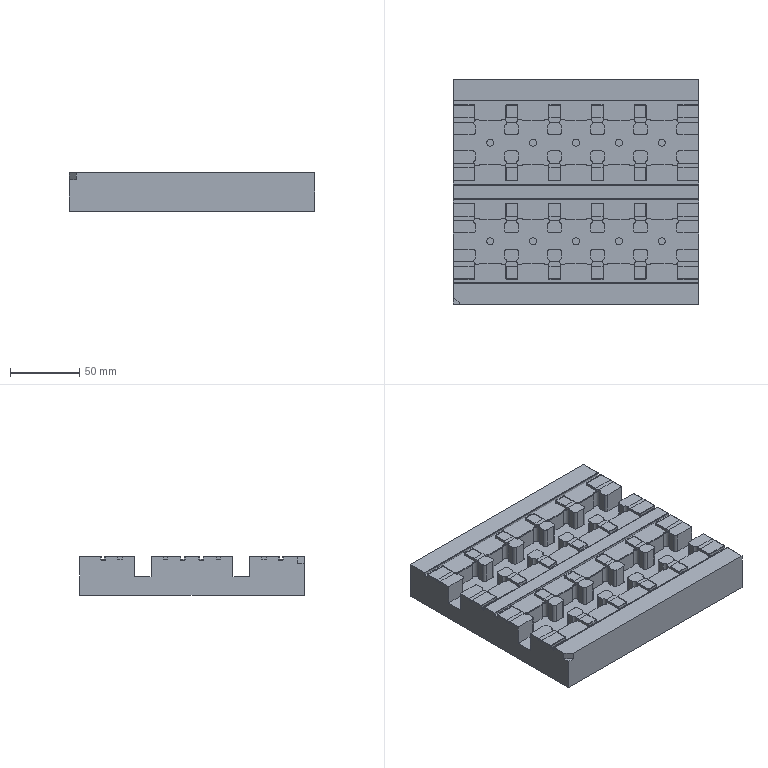NC program | NX | posted by the shop | part box 177 x 162 x 28 mm
Lines 20888 to 21819 of 240480:
N5 T05 M06
(D4  D=4. R=0. H=05 ce=0.02 di=0.05)
(D.N=05 MAX_Z=45. MIN_Z=13.55 Time=44.81M)
T04
G00 G90 G54 X-69.134 Y-48.309 M03 S4000
G43 H05 Z43.
M08
Z28.503
G01 X-69.145 Y-48.308 Z28.405 F1200.
X-69.177 Y-48.307 Z28.318
X-69.229 Y-48.308 Z28.241
X-69.3 Y-48.314 Z28.174
X-69.387 Y-48.328 Z28.115
X-69.49 Y-48.352 Z28.065
X-69.606 Y-48.389 Z28.023
X-69.735 Y-48.44 Z27.988
X-69.875 Y-48.51 Z27.96
X-70.025 Y-48.599 Z27.938
X-70.182 Y-48.712 Z27.922
X-70.346 Y-48.849 Z27.911
X-70.515 Y-49.015 Z27.905
X-70.687 Y-49.211 Z27.903
G02 X-71.571 Y-49.834 I-1.563 J1.28 F1500.
G03 X-71.757 Y-50.097 I.094 J-.264
G01 X-71.753 Y-50.146
G02 X-71.722 Y-50.5 I-1.989 J-.354
X-72.278 Y-51.892 I-2.02 J0.0
X-71.54 Y-53.011 I-1.222 J-1.608
G01 X-71.493 Y-53.158
X-71.436 Y-53.27 Z27.902
X-71.369 Y-53.348 Z27.901
X-71.295 Y-53.395 Z27.9
X-71.214 Y-53.412 Z27.899
X-71.127 Y-53.402 Z27.897
X-71.037 Y-53.366 Z27.895
X-70.942 Y-53.307 Z27.893
X-70.846 Y-53.228 Z27.89
X-70.749 Y-53.129 Z27.888
X-70.652 Y-53.013 Z27.885
X-70.557 Y-52.883 Z27.882
X-70.464 Y-52.74 Z27.879
X-70.376 Y-52.586 Z27.876
X-70.213 Y-52.255 Z27.87
X-70.073 Y-51.898 Z27.864
X-69.957 Y-51.524 Z27.857
X-69.868 Y-51.142 Z27.851
X-69.809 Y-50.759 Z27.844
X-69.78 Y-50.383 Z27.838
X-69.785 Y-50.023 Z27.832
X-69.8 Y-49.852 Z27.829
X-69.825 Y-49.689 Z27.826
X-69.857 Y-49.537 Z27.823
X-69.898 Y-49.398 Z27.82
X-69.946 Y-49.274 Z27.818
X-70.002 Y-49.167 Z27.816
X-70.065 Y-49.08 Z27.813
X-70.136 Y-49.015 Z27.811
X-70.213 Y-48.974 Z27.81
X-70.296 Y-48.959 Z27.808
X-70.385 Y-48.973 Z27.807
X-70.48 Y-49.019 Z27.806
X-70.581 Y-49.097
X-70.687 Y-49.211
G02 X-71.571 Y-49.834 I-1.563 J1.28
G03 X-71.757 Y-50.097 I.094 J-.264
G01 X-71.753 Y-50.146
G02 X-71.722 Y-50.5 I-1.989 J-.354
X-72.278 Y-51.892 I-2.02 J0.0
X-71.54 Y-53.011 I-1.222 J-1.608
G01 X-71.493 Y-53.158 Z27.805
X-71.436 Y-53.27
X-71.369 Y-53.348 Z27.804
X-71.295 Y-53.395 Z27.803
X-71.214 Y-53.412 Z27.801
X-71.127 Y-53.402 Z27.8
X-71.037 Y-53.366 Z27.798
X-70.942 Y-53.307 Z27.796
X-70.846 Y-53.228 Z27.793
X-70.749 Y-53.129 Z27.791
X-70.652 Y-53.013 Z27.788
X-70.557 Y-52.883 Z27.785
X-70.464 Y-52.74 Z27.782
X-70.376 Y-52.586 Z27.779
X-70.213 Y-52.255 Z27.773
X-70.073 Y-51.898 Z27.767
X-69.957 Y-51.524 Z27.76
X-69.868 Y-51.142 Z27.754
X-69.809 Y-50.759 Z27.747
X-69.78 Y-50.383 Z27.741
X-69.785 Y-50.023 Z27.735
X-69.8 Y-49.852 Z27.732
X-69.825 Y-49.689 Z27.729
X-69.857 Y-49.537 Z27.726
X-69.898 Y-49.398 Z27.723
X-69.946 Y-49.274 Z27.721
X-70.002 Y-49.167 Z27.718
X-70.065 Y-49.08 Z27.716
X-70.136 Y-49.015 Z27.714
X-70.213 Y-48.974 Z27.713
X-70.296 Y-48.959 Z27.711
X-70.385 Y-48.973 Z27.71
X-70.48 Y-49.019 Z27.709
X-70.581 Y-49.097
X-70.687 Y-49.211 Z27.708
G02 X-71.571 Y-49.834 I-1.563 J1.28
G03 X-71.757 Y-50.097 I.094 J-.264
G01 X-71.753 Y-50.146
G02 X-71.722 Y-50.5 I-1.989 J-.354
X-72.278 Y-51.892 I-2.02 J0.0
X-71.54 Y-53.011 I-1.222 J-1.608
G01 X-71.493 Y-53.158
X-71.436 Y-53.27
X-71.369 Y-53.348 Z27.707
X-71.295 Y-53.395 Z27.706
X-71.214 Y-53.412 Z27.704
X-71.127 Y-53.402 Z27.702
X-71.037 Y-53.366 Z27.7
X-70.942 Y-53.307 Z27.698
X-70.846 Y-53.228 Z27.696
X-70.749 Y-53.129 Z27.693
X-70.652 Y-53.013 Z27.691
X-70.557 Y-52.883 Z27.688
X-70.464 Y-52.74 Z27.685
X-70.376 Y-52.586 Z27.682
X-70.213 Y-52.255 Z27.676
X-70.073 Y-51.898 Z27.669
X-69.957 Y-51.524 Z27.663
X-69.868 Y-51.142 Z27.656
X-69.809 Y-50.759 Z27.65
X-69.78 Y-50.383 Z27.644
X-69.785 Y-50.023 Z27.637
X-69.8 Y-49.852 Z27.634
X-69.825 Y-49.689 Z27.632
X-69.857 Y-49.537 Z27.629
X-69.898 Y-49.398 Z27.626
X-69.946 Y-49.274 Z27.623
X-70.002 Y-49.167 Z27.621
X-70.065 Y-49.08 Z27.619
X-70.136 Y-49.015 Z27.617
X-70.213 Y-48.974 Z27.615
X-70.296 Y-48.959 Z27.614
X-70.385 Y-48.973 Z27.613
X-70.48 Y-49.019 Z27.612
X-70.581 Y-49.097 Z27.611
X-70.687 Y-49.211
G02 X-71.571 Y-49.834 I-1.563 J1.28
G03 X-71.757 Y-50.097 I.094 J-.264
G01 X-71.753 Y-50.146
G02 X-71.722 Y-50.5 I-1.989 J-.354
X-72.278 Y-51.892 I-2.02 J0.0
X-71.54 Y-53.011 I-1.222 J-1.608
G01 X-71.493 Y-53.158
X-71.436 Y-53.27 Z27.61
X-71.369 Y-53.348
X-71.295 Y-53.395 Z27.608
X-71.214 Y-53.412 Z27.607
X-71.127 Y-53.402 Z27.605
X-71.037 Y-53.366 Z27.603
X-70.942 Y-53.307 Z27.601
X-70.846 Y-53.228 Z27.599
X-70.749 Y-53.129 Z27.596
X-70.652 Y-53.013 Z27.594
X-70.557 Y-52.883 Z27.591
X-70.464 Y-52.74 Z27.588
X-70.376 Y-52.586 Z27.585
X-70.213 Y-52.255 Z27.579
X-70.073 Y-51.898 Z27.572
X-69.957 Y-51.524 Z27.566
X-69.868 Y-51.142 Z27.559
X-69.809 Y-50.759 Z27.553
X-69.78 Y-50.383 Z27.546
X-69.785 Y-50.023 Z27.54
X-69.8 Y-49.852 Z27.537
X-69.825 Y-49.689 Z27.534
X-69.857 Y-49.537 Z27.531
X-69.898 Y-49.398 Z27.529
X-69.946 Y-49.274 Z27.526
X-70.002 Y-49.167 Z27.524
X-70.065 Y-49.08 Z27.522
X-70.136 Y-49.015 Z27.52
X-70.213 Y-48.974 Z27.518
X-70.296 Y-48.959 Z27.517
X-70.385 Y-48.973 Z27.515
X-70.48 Y-49.019
X-70.581 Y-49.097 Z27.514
X-70.687 Y-49.211
G02 X-71.571 Y-49.834 I-1.563 J1.28
G03 X-71.757 Y-50.097 I.094 J-.264
G01 X-71.753 Y-50.146
G02 X-71.722 Y-50.5 I-1.989 J-.354
X-72.278 Y-51.892 I-2.02 J0.0
X-71.54 Y-53.011 I-1.222 J-1.608
G01 X-71.493 Y-53.158
X-71.436 Y-53.27 Z27.513
X-71.369 Y-53.348 Z27.512
X-71.295 Y-53.395 Z27.511
X-71.214 Y-53.412 Z27.51
X-71.127 Y-53.402 Z27.508
X-71.037 Y-53.366 Z27.506
X-70.942 Y-53.307 Z27.504
X-70.846 Y-53.228 Z27.502
X-70.749 Y-53.129 Z27.499
X-70.652 Y-53.013 Z27.496
X-70.557 Y-52.883 Z27.493
X-70.464 Y-52.74 Z27.491
X-70.376 Y-52.586 Z27.488
X-70.213 Y-52.255 Z27.481
X-70.073 Y-51.898 Z27.475
X-69.957 Y-51.524 Z27.469
X-69.868 Y-51.142 Z27.462
X-69.809 Y-50.759 Z27.456
X-69.78 Y-50.383 Z27.449
X-69.785 Y-50.023 Z27.443
X-69.8 Y-49.852 Z27.44
X-69.825 Y-49.689 Z27.437
X-69.857 Y-49.537 Z27.434
X-69.898 Y-49.398 Z27.432
X-69.946 Y-49.274 Z27.429
X-70.002 Y-49.167 Z27.427
X-70.065 Y-49.08 Z27.425
X-70.136 Y-49.015 Z27.423
X-70.213 Y-48.974 Z27.421
X-70.296 Y-48.959 Z27.419
X-70.385 Y-48.973 Z27.418
X-70.48 Y-49.019 Z27.417
X-70.581 Y-49.097
X-70.687 Y-49.211
G02 X-71.571 Y-49.834 I-1.563 J1.28
G03 X-71.757 Y-50.097 I.094 J-.264
G01 X-71.753 Y-50.146
G02 X-71.722 Y-50.5 I-1.989 J-.354
X-72.278 Y-51.892 I-2.02 J0.0
X-71.54 Y-53.011 I-1.222 J-1.608
G01 X-71.493 Y-53.158 Z27.416
X-71.436 Y-53.27
X-71.369 Y-53.348 Z27.415
X-71.295 Y-53.395 Z27.414
X-71.214 Y-53.412 Z27.412
X-71.127 Y-53.402 Z27.411
X-71.037 Y-53.366 Z27.409
X-70.942 Y-53.307 Z27.407
X-70.846 Y-53.228 Z27.404
X-70.749 Y-53.129 Z27.402
X-70.652 Y-53.013 Z27.399
X-70.557 Y-52.883 Z27.396
X-70.464 Y-52.74 Z27.393
X-70.376 Y-52.586 Z27.39
X-70.213 Y-52.255 Z27.384
X-70.073 Y-51.898 Z27.378
X-69.957 Y-51.524 Z27.371
X-69.868 Y-51.142 Z27.365
X-69.809 Y-50.759 Z27.358
X-69.78 Y-50.383 Z27.352
X-69.785 Y-50.023 Z27.346
X-69.8 Y-49.852 Z27.343
X-69.825 Y-49.689 Z27.34
X-69.857 Y-49.537 Z27.337
X-69.898 Y-49.398 Z27.334
X-69.946 Y-49.274 Z27.332
X-70.002 Y-49.167 Z27.329
X-70.065 Y-49.08 Z27.327
X-70.136 Y-49.015 Z27.325
X-70.213 Y-48.974 Z27.324
X-70.296 Y-48.959 Z27.322
X-70.385 Y-48.973 Z27.321
X-70.48 Y-49.019 Z27.32
X-70.581 Y-49.097
X-70.687 Y-49.211 Z27.319
G02 X-71.571 Y-49.834 I-1.563 J1.28
G03 X-71.757 Y-50.097 I.094 J-.264
G01 X-71.753 Y-50.146
G02 X-71.722 Y-50.5 I-1.989 J-.354
X-72.278 Y-51.892 I-2.02 J0.0
X-71.54 Y-53.011 I-1.222 J-1.608
G01 X-71.493 Y-53.158
X-71.436 Y-53.27
X-71.369 Y-53.348 Z27.318
X-71.295 Y-53.395 Z27.317
X-71.214 Y-53.412 Z27.315
X-71.127 Y-53.402 Z27.314
X-71.037 Y-53.366 Z27.312
X-70.942 Y-53.307 Z27.309
X-70.846 Y-53.228 Z27.307
X-70.749 Y-53.129 Z27.305
X-70.652 Y-53.013 Z27.302
X-70.557 Y-52.883 Z27.299
X-70.464 Y-52.74 Z27.296
X-70.376 Y-52.586 Z27.293
X-70.213 Y-52.255 Z27.287
X-70.073 Y-51.898 Z27.281
X-69.957 Y-51.524 Z27.274
X-69.868 Y-51.142 Z27.268
X-69.809 Y-50.759 Z27.261
X-69.78 Y-50.383 Z27.255
X-69.785 Y-50.023 Z27.249
X-69.8 Y-49.852 Z27.246
X-69.825 Y-49.689 Z27.243
X-69.857 Y-49.537 Z27.24
X-69.898 Y-49.398 Z27.237
X-69.946 Y-49.274 Z27.235
X-70.002 Y-49.167 Z27.232
X-70.065 Y-49.08 Z27.23
X-70.136 Y-49.015 Z27.228
X-70.213 Y-48.974 Z27.226
X-70.296 Y-48.959 Z27.225
X-70.385 Y-48.973 Z27.224
X-70.48 Y-49.019 Z27.223
X-70.581 Y-49.097 Z27.222
X-70.687 Y-49.211
G02 X-71.571 Y-49.834 I-1.563 J1.28
G03 X-71.757 Y-50.097 I.094 J-.264
G01 X-71.753 Y-50.146
G02 X-71.722 Y-50.5 I-1.989 J-.354
X-72.278 Y-51.892 I-2.02 J0.0
X-71.54 Y-53.011 I-1.222 J-1.608
G01 X-71.493 Y-53.158
X-71.436 Y-53.27
X-71.369 Y-53.348 Z27.221
X-71.295 Y-53.395 Z27.219
X-71.214 Y-53.412 Z27.218
X-71.127 Y-53.402 Z27.216
X-71.037 Y-53.366 Z27.214
X-70.942 Y-53.307 Z27.212
X-70.846 Y-53.228 Z27.21
X-70.749 Y-53.129 Z27.207
X-70.652 Y-53.013 Z27.205
X-70.557 Y-52.883 Z27.202
X-70.464 Y-52.74 Z27.199
X-70.376 Y-52.586 Z27.196
X-70.213 Y-52.255 Z27.19
X-70.073 Y-51.898 Z27.183
X-69.957 Y-51.524 Z27.177
X-69.868 Y-51.142 Z27.17
X-69.809 Y-50.759 Z27.164
X-69.78 Y-50.383 Z27.158
X-69.785 Y-50.023 Z27.151
X-69.8 Y-49.852 Z27.148
X-69.825 Y-49.689 Z27.145
X-69.857 Y-49.537 Z27.143
X-69.898 Y-49.398 Z27.14
X-69.946 Y-49.274 Z27.137
X-70.002 Y-49.167 Z27.135
X-70.065 Y-49.08 Z27.133
X-70.136 Y-49.015 Z27.131
X-70.213 Y-48.974 Z27.129
X-70.296 Y-48.959 Z27.128
X-70.385 Y-48.973 Z27.127
X-70.48 Y-49.019 Z27.126
X-70.581 Y-49.097 Z27.125
X-70.687 Y-49.211
G02 X-71.571 Y-49.834 I-1.563 J1.28
G03 X-71.757 Y-50.097 I.094 J-.264
G01 X-71.753 Y-50.146
G02 X-71.722 Y-50.5 I-1.989 J-.354
X-72.278 Y-51.892 I-2.02 J0.0
X-71.54 Y-53.011 I-1.222 J-1.608
G01 X-71.493 Y-53.158
X-71.436 Y-53.27 Z27.124
X-71.369 Y-53.348 Z27.123
X-71.295 Y-53.395 Z27.122
X-71.214 Y-53.412 Z27.121
X-71.127 Y-53.402 Z27.119
X-71.037 Y-53.366 Z27.117
X-70.942 Y-53.307 Z27.115
X-70.846 Y-53.228 Z27.113
X-70.749 Y-53.129 Z27.11
X-70.652 Y-53.013 Z27.107
X-70.557 Y-52.883 Z27.105
X-70.464 Y-52.74 Z27.102
X-70.376 Y-52.586 Z27.099
X-70.213 Y-52.255 Z27.092
X-70.073 Y-51.898 Z27.086
X-69.957 Y-51.524 Z27.08
X-69.868 Y-51.142 Z27.073
X-69.809 Y-50.759 Z27.067
X-69.78 Y-50.383 Z27.06
X-69.785 Y-50.023 Z27.054
X-69.8 Y-49.852 Z27.051
X-69.825 Y-49.689 Z27.048
X-69.857 Y-49.537 Z27.045
X-69.898 Y-49.398 Z27.043
X-69.946 Y-49.274 Z27.04
X-70.002 Y-49.167 Z27.038
X-70.065 Y-49.08 Z27.036
X-70.136 Y-49.015 Z27.034
X-70.213 Y-48.974 Z27.032
X-70.296 Y-48.959 Z27.031
X-70.385 Y-48.973 Z27.029
X-70.48 Y-49.019 Z27.028
X-70.581 Y-49.097
X-70.687 Y-49.211
G02 X-71.571 Y-49.834 I-1.563 J1.28
G03 X-71.757 Y-50.097 I.094 J-.264
G01 X-71.753 Y-50.146
G02 X-71.722 Y-50.5 I-1.989 J-.354
X-72.278 Y-51.892 I-2.02 J0.0
X-71.54 Y-53.011 I-1.222 J-1.608
G01 X-71.493 Y-53.158
X-71.436 Y-53.27 Z27.027
X-71.369 Y-53.348 Z27.026
X-71.295 Y-53.395 Z27.025
X-71.214 Y-53.412 Z27.024
X-71.127 Y-53.402 Z27.022
X-71.037 Y-53.366 Z27.02
X-70.942 Y-53.307 Z27.018
X-70.846 Y-53.228 Z27.015
X-70.749 Y-53.129 Z27.013
X-70.652 Y-53.013 Z27.01
X-70.557 Y-52.883 Z27.007
X-70.464 Y-52.74 Z27.004
X-70.376 Y-52.586 Z27.001
X-70.213 Y-52.255 Z26.995
X-70.073 Y-51.898 Z26.989
X-69.957 Y-51.524 Z26.982
X-69.868 Y-51.142 Z26.976
X-69.809 Y-50.759 Z26.969
X-69.78 Y-50.383 Z26.963
X-69.785 Y-50.023 Z26.957
X-69.8 Y-49.852 Z26.954
X-69.825 Y-49.689 Z26.951
X-69.857 Y-49.537 Z26.948
X-69.898 Y-49.398 Z26.945
X-69.946 Y-49.274 Z26.943
X-70.002 Y-49.167 Z26.941
X-70.065 Y-49.08 Z26.938
X-70.136 Y-49.015 Z26.936
X-70.213 Y-48.974 Z26.935
X-70.296 Y-48.959 Z26.933
X-70.385 Y-48.973 Z26.932
X-70.48 Y-49.019 Z26.931
X-70.581 Y-49.097
X-70.687 Y-49.211
G02 X-71.571 Y-49.834 I-1.563 J1.28
G03 X-71.757 Y-50.097 I.094 J-.264
G01 X-71.753 Y-50.146
G02 X-71.722 Y-50.5 I-1.989 J-.354
X-72.278 Y-51.892 I-2.02 J0.0
X-71.54 Y-53.011 I-1.222 J-1.608
G01 X-71.493 Y-53.158 Z26.93
X-71.436 Y-53.27
X-71.369 Y-53.348 Z26.929
X-71.295 Y-53.395 Z26.928
X-71.214 Y-53.412 Z26.926
X-71.127 Y-53.402 Z26.925
X-71.037 Y-53.366 Z26.923
X-70.942 Y-53.307 Z26.921
X-70.846 Y-53.228 Z26.918
X-70.749 Y-53.129 Z26.916
X-70.652 Y-53.013 Z26.913
X-70.557 Y-52.883 Z26.91
X-70.464 Y-52.74 Z26.907
X-70.376 Y-52.586 Z26.904
X-70.213 Y-52.255 Z26.898
X-70.073 Y-51.898 Z26.892
X-69.957 Y-51.524 Z26.885
X-69.868 Y-51.142 Z26.879
X-69.809 Y-50.759 Z26.872
X-69.78 Y-50.383 Z26.866
X-69.785 Y-50.023 Z26.86
X-69.8 Y-49.852 Z26.857
X-69.825 Y-49.689 Z26.854
X-69.857 Y-49.537 Z26.851
X-69.898 Y-49.398 Z26.848
X-69.946 Y-49.274 Z26.846
X-70.002 Y-49.167 Z26.843
X-70.065 Y-49.08 Z26.841
X-70.136 Y-49.015 Z26.839
X-70.213 Y-48.974 Z26.838
X-70.296 Y-48.959 Z26.836
X-70.385 Y-48.973 Z26.835
X-70.48 Y-49.019 Z26.834
X-70.581 Y-49.097
X-70.687 Y-49.211 Z26.833
G02 X-71.571 Y-49.834 I-1.563 J1.28
G03 X-71.757 Y-50.097 I.094 J-.264
G01 X-71.753 Y-50.146
G02 X-71.722 Y-50.5 I-1.989 J-.354
X-72.278 Y-51.892 I-2.02 J0.0
X-71.54 Y-53.011 I-1.222 J-1.608
G01 X-71.493 Y-53.158
X-71.436 Y-53.27
X-71.369 Y-53.348 Z26.832
X-71.295 Y-53.395 Z26.831
X-71.214 Y-53.412 Z26.829
X-71.127 Y-53.402 Z26.827
X-71.037 Y-53.366 Z26.825
X-70.942 Y-53.307 Z26.823
X-70.846 Y-53.228 Z26.821
X-70.749 Y-53.129 Z26.818
X-70.652 Y-53.013 Z26.816
X-70.557 Y-52.883 Z26.813
X-70.464 Y-52.74 Z26.81
X-70.376 Y-52.586 Z26.807
X-70.213 Y-52.255 Z26.801
X-70.073 Y-51.898 Z26.794
X-69.957 Y-51.524 Z26.788
X-69.868 Y-51.142 Z26.781
X-69.809 Y-50.759 Z26.775
X-69.78 Y-50.383 Z26.769
X-69.785 Y-50.023 Z26.762
X-69.8 Y-49.852 Z26.759
X-69.825 Y-49.689 Z26.757
X-69.857 Y-49.537 Z26.754
X-69.898 Y-49.398 Z26.751
X-69.946 Y-49.274 Z26.748
X-70.002 Y-49.167 Z26.746
X-70.065 Y-49.08 Z26.744
X-70.136 Y-49.015 Z26.742
X-70.213 Y-48.974 Z26.74
X-70.296 Y-48.959 Z26.739
X-70.385 Y-48.973 Z26.738
X-70.48 Y-49.019 Z26.737
X-70.581 Y-49.097 Z26.736
X-70.687 Y-49.211
G02 X-71.571 Y-49.834 I-1.563 J1.28
G03 X-71.757 Y-50.097 I.094 J-.264
G01 X-71.753 Y-50.146
G02 X-71.722 Y-50.5 I-1.989 J-.354
X-72.278 Y-51.892 I-2.02 J0.0
X-71.54 Y-53.011 I-1.222 J-1.608
G01 X-71.493 Y-53.158
X-71.436 Y-53.27 Z26.735
X-71.369 Y-53.348
X-71.295 Y-53.395 Z26.733
X-71.214 Y-53.412 Z26.732
X-71.127 Y-53.402 Z26.73
X-71.037 Y-53.366 Z26.728
X-70.942 Y-53.307 Z26.726
X-70.846 Y-53.228 Z26.724
X-70.749 Y-53.129 Z26.721
X-70.652 Y-53.013 Z26.719
X-70.557 Y-52.883 Z26.716
X-70.464 Y-52.74 Z26.713
X-70.376 Y-52.586 Z26.71
X-70.213 Y-52.255 Z26.704
X-70.073 Y-51.898 Z26.697
X-69.957 Y-51.524 Z26.691
X-69.868 Y-51.142 Z26.684
X-69.809 Y-50.759 Z26.678
X-69.78 Y-50.383 Z26.671
X-69.785 Y-50.023 Z26.665
X-69.8 Y-49.852 Z26.662
X-69.825 Y-49.689 Z26.659
X-69.857 Y-49.537 Z26.656
X-69.898 Y-49.398 Z26.654
X-69.946 Y-49.274 Z26.651
X-70.002 Y-49.167 Z26.649
X-70.065 Y-49.08 Z26.647
X-70.136 Y-49.015 Z26.645
X-70.213 Y-48.974 Z26.643
X-70.296 Y-48.959 Z26.642
X-70.385 Y-48.973 Z26.64
X-70.48 Y-49.019
X-70.581 Y-49.097 Z26.639
X-70.687 Y-49.211
G02 X-71.571 Y-49.834 I-1.563 J1.28
G03 X-71.757 Y-50.097 I.094 J-.264
G01 X-71.753 Y-50.146
G02 X-71.722 Y-50.5 I-1.989 J-.354
X-72.278 Y-51.892 I-2.02 J0.0
X-71.54 Y-53.011 I-1.222 J-1.608
G01 X-71.493 Y-53.158
X-71.436 Y-53.27 Z26.638
X-71.369 Y-53.348 Z26.637
X-71.295 Y-53.395 Z26.636
X-71.214 Y-53.412 Z26.635
X-71.127 Y-53.402 Z26.633
X-71.037 Y-53.366 Z26.631
X-70.942 Y-53.307 Z26.629
X-70.846 Y-53.228 Z26.627
X-70.749 Y-53.129 Z26.624
X-70.652 Y-53.013 Z26.621
X-70.557 Y-52.883 Z26.618
X-70.464 Y-52.74 Z26.616
X-70.376 Y-52.586 Z26.613
X-70.213 Y-52.255 Z26.606
X-70.073 Y-51.898 Z26.6
X-69.957 Y-51.524 Z26.594
X-69.868 Y-51.142 Z26.587
X-69.809 Y-50.759 Z26.581
X-69.78 Y-50.383 Z26.574
X-69.785 Y-50.023 Z26.568
X-69.8 Y-49.852 Z26.565
X-69.825 Y-49.689 Z26.562
X-69.857 Y-49.537 Z26.559
X-69.898 Y-49.398 Z26.557
X-69.946 Y-49.274 Z26.554
X-70.002 Y-49.167 Z26.552
X-70.065 Y-49.08 Z26.55
X-70.136 Y-49.015 Z26.548
X-70.213 Y-48.974 Z26.546
X-70.296 Y-48.959 Z26.544
X-70.385 Y-48.973 Z26.543
X-70.48 Y-49.019 Z26.542
X-70.581 Y-49.097
X-70.687 Y-49.211
G02 X-71.571 Y-49.834 I-1.563 J1.28
G03 X-71.757 Y-50.097 I.094 J-.264
G01 X-71.753 Y-50.146
G02 X-71.722 Y-50.5 I-1.989 J-.354
X-72.278 Y-51.892 I-2.02 J0.0
X-71.54 Y-53.011 I-1.222 J-1.608
G01 X-71.493 Y-53.158 Z26.541
X-71.436 Y-53.27
X-71.369 Y-53.348 Z26.54
X-71.295 Y-53.395 Z26.539
X-71.214 Y-53.412 Z26.537
X-71.127 Y-53.402 Z26.536
X-71.037 Y-53.366 Z26.534
X-70.942 Y-53.307 Z26.532
X-70.846 Y-53.228 Z26.529
X-70.749 Y-53.129 Z26.527
X-70.652 Y-53.013 Z26.524
X-70.557 Y-52.883 Z26.521
X-70.464 Y-52.74 Z26.518
X-70.376 Y-52.586 Z26.515
X-70.213 Y-52.255 Z26.509
X-70.073 Y-51.898 Z26.503
X-69.957 Y-51.524 Z26.496
X-69.868 Y-51.142 Z26.49
X-69.809 Y-50.759 Z26.483
X-69.78 Y-50.383 Z26.477
X-69.785 Y-50.023 Z26.471
X-69.8 Y-49.852 Z26.468
X-69.825 Y-49.689 Z26.465
X-69.857 Y-49.537 Z26.462
X-69.898 Y-49.398 Z26.459
X-69.946 Y-49.274 Z26.457
X-70.002 Y-49.167 Z26.454
X-70.065 Y-49.08 Z26.452
X-70.136 Y-49.015 Z26.45
X-70.213 Y-48.974 Z26.449
X-70.296 Y-48.959 Z26.447
X-70.385 Y-48.973 Z26.446
X-70.48 Y-49.019 Z26.445
X-70.581 Y-49.097
X-70.687 Y-49.211 Z26.444
G02 X-71.571 Y-49.834 I-1.563 J1.28
G03 X-71.757 Y-50.097 I.094 J-.264
G01 X-71.753 Y-50.146
G02 X-71.722 Y-50.5 I-1.989 J-.354
X-72.278 Y-51.892 I-2.02 J0.0
X-71.54 Y-53.011 I-1.222 J-1.608
G01 X-71.493 Y-53.158
X-71.436 Y-53.27
X-71.369 Y-53.348 Z26.443
X-71.295 Y-53.395 Z26.442
X-71.214 Y-53.412 Z26.44
X-71.127 Y-53.402 Z26.439
X-71.037 Y-53.366 Z26.437
X-70.942 Y-53.307 Z26.434
X-70.846 Y-53.228 Z26.432
X-70.749 Y-53.129 Z26.43
X-70.652 Y-53.013 Z26.427
X-70.557 Y-52.883 Z26.424
X-70.464 Y-52.74 Z26.421
X-70.376 Y-52.586 Z26.418
X-70.213 Y-52.255 Z26.412
X-70.073 Y-51.898 Z26.406
X-69.957 Y-51.524 Z26.399
X-69.868 Y-51.142 Z26.393
X-69.809 Y-50.759 Z26.386
X-69.78 Y-50.383 Z26.38
X-69.785 Y-50.023 Z26.374
X-69.8 Y-49.852 Z26.371
X-69.825 Y-49.689 Z26.368
X-69.857 Y-49.537 Z26.365
X-69.898 Y-49.398 Z26.362
X-69.946 Y-49.274 Z26.36
X-70.002 Y-49.167 Z26.357
X-70.065 Y-49.08 Z26.355
X-70.136 Y-49.015 Z26.353
X-70.213 Y-48.974 Z26.351
X-70.296 Y-48.959 Z26.35
X-70.385 Y-48.973 Z26.349
X-70.48 Y-49.019 Z26.348
X-70.581 Y-49.097 Z26.347
X-70.687 Y-49.211
G02 X-71.571 Y-49.834 I-1.563 J1.28
G03 X-71.757 Y-50.097 I.094 J-.264
G01 X-71.753 Y-50.146
G02 X-71.722 Y-50.5 I-1.989 J-.354
X-72.278 Y-51.892 I-2.02 J0.0
X-71.54 Y-53.011 I-1.222 J-1.608
G01 X-71.493 Y-53.158
X-71.436 Y-53.27
X-71.369 Y-53.348 Z26.346
X-71.295 Y-53.395 Z26.344
X-71.214 Y-53.412 Z26.343
X-71.127 Y-53.402 Z26.341
X-71.037 Y-53.366 Z26.339
X-70.942 Y-53.307 Z26.337
X-70.846 Y-53.228 Z26.335
X-70.749 Y-53.129 Z26.332
X-70.652 Y-53.013 Z26.33
X-70.557 Y-52.883 Z26.327
X-70.464 Y-52.74 Z26.324
X-70.376 Y-52.586 Z26.321
X-70.213 Y-52.255 Z26.315
X-70.073 Y-51.898 Z26.308
X-69.957 Y-51.524 Z26.302
X-69.868 Y-51.142 Z26.295
X-69.809 Y-50.759 Z26.289
X-69.78 Y-50.383 Z26.283
X-69.785 Y-50.023 Z26.276
X-69.8 Y-49.852 Z26.273
X-69.825 Y-49.689 Z26.27
X-69.857 Y-49.537 Z26.268
X-69.898 Y-49.398 Z26.265
X-69.946 Y-49.274 Z26.262
X-70.002 Y-49.167 Z26.26
X-70.065 Y-49.08 Z26.258
X-70.136 Y-49.015 Z26.256
X-70.213 Y-48.974 Z26.254
X-70.296 Y-48.959 Z26.253
X-70.385 Y-48.973 Z26.252
X-70.48 Y-49.019 Z26.251
X-70.581 Y-49.097 Z26.25
X-70.687 Y-49.211
G02 X-71.571 Y-49.834 I-1.563 J1.28
G03 X-71.757 Y-50.097 I.094 J-.264
G01 X-71.753 Y-50.146
G02 X-71.722 Y-50.5 I-1.989 J-.354
X-72.278 Y-51.892 I-2.02 J0.0
X-71.54 Y-53.011 I-1.222 J-1.608
G01 X-71.449 Y-53.352 Z26.262
X-71.344 Y-53.708 Z26.297
X-71.233 Y-54.076 Z26.35
X-71.121 Y-54.453 Z26.42
X-71.016 Y-54.834 Z26.503
X-70.922 Y-55.217 Z26.597
X-70.846 Y-55.598 Z26.698
X-70.788 Y-56.037 Z26.821
X-70.761 Y-56.472 Z26.948
X-70.765 Y-56.909 Z27.076
X-70.797 Y-57.35 Z27.205
X-70.857 Y-57.798 Z27.332
X-70.942 Y-58.259 Z27.455
X-71.101 Y-58.938 Z27.617
X-71.205 Y-59.367 Z27.707
X-71.362 Y-60.047 Z27.825
X-71.424 Y-60.389 Z27.867
X-71.465 Y-60.717 Z27.893
X-71.48 Y-61.027 Z27.903
Y-63.2
G02 X-71.734 Y-64.18 I-2.02 J0.0
G01 X-68.327
X-68.169 Y-64.168
X-68.038 Y-64.132 Z27.902
X-67.933 Y-64.076 Z27.901
X-67.851 Y-64. Z27.9
X-67.792 Y-63.907 Z27.899
X-67.755 Y-63.798 Z27.897
X-67.737 Y-63.676 Z27.895
Y-63.542 Z27.893
X-67.755 Y-63.399 Z27.89
X-67.788 Y-63.248 Z27.888
X-67.835 Y-63.091 Z27.885
X-67.896 Y-62.93 Z27.882
X-67.967 Y-62.768 Z27.879
X-68.049 Y-62.605 Z27.876
X-68.24 Y-62.286 Z27.87
X-68.461 Y-61.978 Z27.864
X-68.71 Y-61.686 Z27.857
X-68.982 Y-61.413 Z27.851
X-69.274 Y-61.164 Z27.844
X-69.582 Y-60.942 Z27.838
X-69.901 Y-60.751 Z27.832
X-70.064 Y-60.669 Z27.829
X-70.227 Y-60.597 Z27.826
X-70.388 Y-60.536 Z27.823
X-70.545 Y-60.489 Z27.82
X-70.696 Y-60.455 Z27.818
X-70.84 Y-60.438 Z27.816
X-70.974 Y-60.437 Z27.813
X-71.097 Y-60.455 Z27.811
X-71.206 Y-60.493 Z27.81
X-71.299 Y-60.552 Z27.808
X-71.375 Y-60.633 Z27.807
X-71.432 Y-60.739 Z27.806
X-71.468 Y-60.869
X-71.48 Y-61.027
Y-63.2
G02 X-71.734 Y-64.18 I-2.02 J0.0
G01 X-68.327
X-68.169 Y-64.168 Z27.805
X-68.038 Y-64.132
X-67.933 Y-64.076 Z27.804
X-67.851 Y-64. Z27.803
X-67.792 Y-63.907 Z27.801
X-67.755 Y-63.798 Z27.8
X-67.737 Y-63.676 Z27.798
Y-63.542 Z27.796
X-67.755 Y-63.399 Z27.793
X-67.788 Y-63.248 Z27.791
X-67.835 Y-63.091 Z27.788
X-67.896 Y-62.93 Z27.785
X-67.967 Y-62.768 Z27.782
X-68.049 Y-62.605 Z27.779
X-68.24 Y-62.286 Z27.773
X-68.461 Y-61.978 Z27.767
X-68.71 Y-61.686 Z27.76
X-68.982 Y-61.413 Z27.754
X-69.274 Y-61.164 Z27.747
X-69.582 Y-60.942 Z27.741
X-69.901 Y-60.751 Z27.735
X-70.064 Y-60.669 Z27.732
X-70.227 Y-60.597 Z27.729
X-70.388 Y-60.536 Z27.726
X-70.545 Y-60.489 Z27.723
X-70.696 Y-60.455 Z27.721
X-70.84 Y-60.438 Z27.718
X-70.974 Y-60.437 Z27.716
X-71.097 Y-60.455 Z27.714
X-71.206 Y-60.493 Z27.713
X-71.299 Y-60.552 Z27.711
X-71.375 Y-60.633 Z27.71
X-71.432 Y-60.739 Z27.709
X-71.468 Y-60.869
X-71.48 Y-61.027 Z27.708
Y-63.2
G02 X-71.734 Y-64.18 I-2.02 J0.0
G01 X-68.327
X-68.169 Y-64.168
X-68.038 Y-64.132
X-67.933 Y-64.076 Z27.707
X-67.851 Y-64. Z27.706
X-67.792 Y-63.907 Z27.704
X-67.755 Y-63.798 Z27.702
X-67.737 Y-63.676 Z27.7
Y-63.542 Z27.698
X-67.755 Y-63.399 Z27.696
X-67.788 Y-63.248 Z27.693
X-67.835 Y-63.091 Z27.691
X-67.896 Y-62.93 Z27.688
X-67.967 Y-62.768 Z27.685
X-68.049 Y-62.605 Z27.682
X-68.24 Y-62.286 Z27.676
X-68.461 Y-61.978 Z27.669
X-68.71 Y-61.686 Z27.663
X-68.982 Y-61.413 Z27.656
X-69.274 Y-61.164 Z27.65
X-69.582 Y-60.942 Z27.644
X-69.901 Y-60.751 Z27.637
X-70.064 Y-60.669 Z27.634
X-70.227 Y-60.597 Z27.632
X-70.388 Y-60.536 Z27.629
X-70.545 Y-60.489 Z27.626
X-70.696 Y-60.455 Z27.623
X-70.84 Y-60.438 Z27.621
X-70.974 Y-60.437 Z27.619
X-71.097 Y-60.455 Z27.617
X-71.206 Y-60.493 Z27.615
X-71.299 Y-60.552 Z27.614
X-71.375 Y-60.633 Z27.613
X-71.432 Y-60.739 Z27.612
X-71.468 Y-60.869 Z27.611
X-71.48 Y-61.027
Y-63.2
G02 X-71.734 Y-64.18 I-2.02 J0.0
G01 X-68.327
X-68.169 Y-64.168
X-68.038 Y-64.132 Z27.61
X-67.933 Y-64.076
X-67.851 Y-64. Z27.608
X-67.792 Y-63.907 Z27.607
X-67.755 Y-63.798 Z27.605
X-67.737 Y-63.676 Z27.603
Y-63.542 Z27.601
X-67.755 Y-63.399 Z27.599
X-67.788 Y-63.248 Z27.596
X-67.835 Y-63.091 Z27.594
X-67.896 Y-62.93 Z27.591
X-67.967 Y-62.768 Z27.588
X-68.049 Y-62.605 Z27.585
X-68.24 Y-62.286 Z27.579
X-68.461 Y-61.978 Z27.572
X-68.71 Y-61.686 Z27.566
X-68.982 Y-61.413 Z27.559
X-69.274 Y-61.164 Z27.553
X-69.582 Y-60.942 Z27.546
X-69.901 Y-60.751 Z27.54
X-70.064 Y-60.669 Z27.537
X-70.227 Y-60.597 Z27.534
X-70.388 Y-60.536 Z27.531
X-70.545 Y-60.489 Z27.529
X-70.696 Y-60.455 Z27.526
X-70.84 Y-60.438 Z27.524
X-70.974 Y-60.437 Z27.522
X-71.097 Y-60.455 Z27.52
X-71.206 Y-60.493 Z27.518
X-71.299 Y-60.552 Z27.517
X-71.375 Y-60.633 Z27.515
X-71.432 Y-60.739
X-71.468 Y-60.869 Z27.514
X-71.48 Y-61.027
Y-63.2
G02 X-71.734 Y-64.18 I-2.02 J0.0
G01 X-68.327
X-68.169 Y-64.168
X-68.038 Y-64.132 Z27.513
X-67.933 Y-64.076 Z27.512
X-67.851 Y-64. Z27.511
X-67.792 Y-63.907 Z27.51
X-67.755 Y-63.798 Z27.508
X-67.737 Y-63.676 Z27.506
Y-63.542 Z27.504
X-67.755 Y-63.399 Z27.502
X-67.788 Y-63.248 Z27.499
X-67.835 Y-63.091 Z27.496
X-67.896 Y-62.93 Z27.493
X-67.967 Y-62.768 Z27.491
X-68.049 Y-62.605 Z27.488
X-68.24 Y-62.286 Z27.481
X-68.461 Y-61.978 Z27.475
X-68.71 Y-61.686 Z27.469
X-68.982 Y-61.413 Z27.462
X-69.274 Y-61.164 Z27.456
X-69.582 Y-60.942 Z27.449
X-69.901 Y-60.751 Z27.443
X-70.064 Y-60.669 Z27.44
X-70.227 Y-60.597 Z27.437
X-70.388 Y-60.536 Z27.434
X-70.545 Y-60.489 Z27.432
X-70.696 Y-60.455 Z27.429
X-70.84 Y-60.438 Z27.427
X-70.974 Y-60.437 Z27.425
X-71.097 Y-60.455 Z27.423
X-71.206 Y-60.493 Z27.421
X-71.299 Y-60.552 Z27.419
X-71.375 Y-60.633 Z27.418
X-71.432 Y-60.739 Z27.417